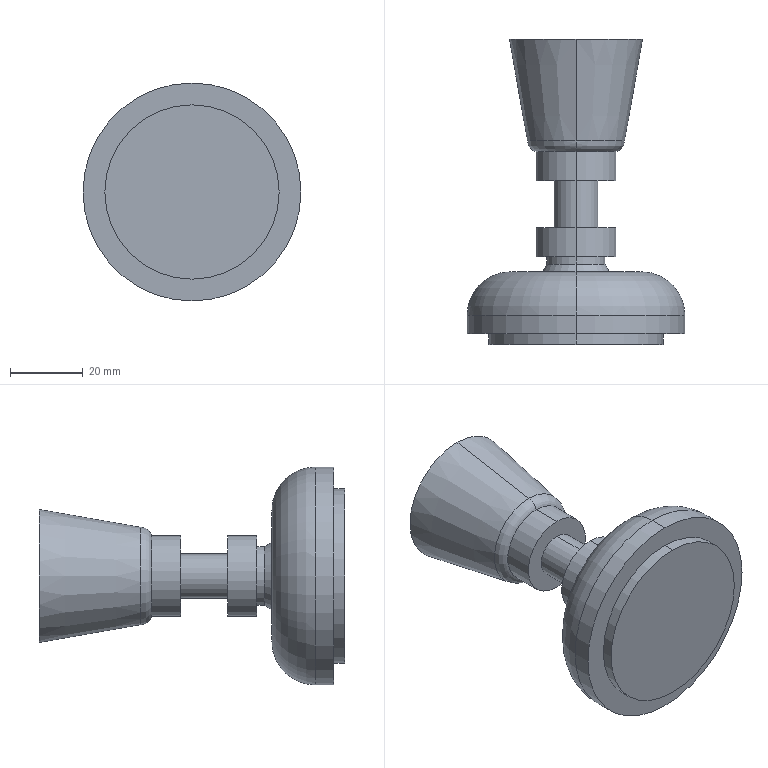Part | SolidWorks | features Revolution 1 | 1 solid | 27 faces | box 60 x 84 x 60 mm | volume 80542 mm3 | cylinder 12 | plane 7 | cone 4 | torus 4 | commonest cylinder face diameters 22.179 x4 12.179 x2 16.179 x2 48 x2 60 x2
STEP:
#1=CARTESIAN_POINT('',(0.,36.531,-13.4));
#2=VERTEX_POINT('',#1);
#3=CARTESIAN_POINT('',(0.,36.531,13.4));
#4=VERTEX_POINT('',#3);
#5=CARTESIAN_POINT('',(0.,36.531,0.));
#6=DIRECTION('',(0.,-1.,0.));
#7=DIRECTION('',(0.,0.,-1.));
#8=AXIS2_PLACEMENT_3D('',#5,#6,#7);
#9=CIRCLE('',#8,13.4);
#10=EDGE_CURVE('',#2,#4,#9,.T.);
#11=ORIENTED_EDGE('',*,*,#10,.F.);
#12=CARTESIAN_POINT('',(0.,64.484,-18.3));
#13=VERTEX_POINT('',#12);
#14=CARTESIAN_POINT('',(0.,36.531,-13.4));
#15=DIRECTION('',(0.,0.985,-0.1727));
#16=VECTOR('',#15,1000.);
#17=LINE('',#14,#16);
#18=EDGE_CURVE('',#2,#13,#17,.T.);
#19=ORIENTED_EDGE('',*,*,#18,.T.);
#20=CARTESIAN_POINT('',(0.,64.484,18.3));
#21=VERTEX_POINT('',#20);
#22=CARTESIAN_POINT('',(0.,64.484,0.));
#23=DIRECTION('',(0.,-1.,0.));
#24=DIRECTION('',(0.,0.,-1.));
#25=AXIS2_PLACEMENT_3D('',#22,#23,#24);
#26=CIRCLE('',#25,18.3);
#27=EDGE_CURVE('',#13,#21,#26,.T.);
#28=ORIENTED_EDGE('',*,*,#27,.T.);
#29=CARTESIAN_POINT('',(0.,36.531,13.4));
#30=DIRECTION('',(0.,0.985,0.1727));
#31=VECTOR('',#30,1000.);
#32=LINE('',#29,#31);
#33=EDGE_CURVE('',#4,#21,#32,.T.);
#34=ORIENTED_EDGE('',*,*,#33,.F.);
#35=EDGE_LOOP('',(#11,#19,#28,#34));
#36=FACE_OUTER_BOUND('',#35,.T.);
#37=CARTESIAN_POINT('',(0.,36.531,0.));
#38=DIRECTION('',(0.,1.,0.));
#39=DIRECTION('',(0.,0.,1.));
#40=AXIS2_PLACEMENT_3D('',#37,#38,#39);
#41=CONICAL_SURFACE('',#40,13.4,0.1735);
#42=ADVANCED_FACE('',(#36),#41,.T.);
#43=ORIENTED_EDGE('',*,*,#10,.T.);
#44=CARTESIAN_POINT('',(0.,33.612,11.09));
#45=VERTEX_POINT('',#44);
#46=CARTESIAN_POINT('',(0.,36.531,10.4));
#47=DIRECTION('',(1.,0.,0.));
#48=DIRECTION('',(0.,0.,-1.));
#49=AXIS2_PLACEMENT_3D('',#46,#47,#48);
#50=CIRCLE('',#49,3.);
#51=EDGE_CURVE('',#4,#45,#50,.T.);
#52=ORIENTED_EDGE('',*,*,#51,.T.);
#53=CARTESIAN_POINT('',(0.,33.612,-11.09));
#54=VERTEX_POINT('',#53);
#55=CARTESIAN_POINT('',(0.,33.612,0.));
#56=DIRECTION('',(0.,-1.,0.));
#57=DIRECTION('',(0.,0.,-1.));
#58=AXIS2_PLACEMENT_3D('',#55,#56,#57);
#59=CIRCLE('',#58,11.09);
#60=EDGE_CURVE('',#54,#45,#59,.T.);
#61=ORIENTED_EDGE('',*,*,#60,.F.);
#62=CARTESIAN_POINT('',(0.,36.531,-10.4));
#63=DIRECTION('',(-1.,0.,0.));
#64=DIRECTION('',(0.,0.,1.));
#65=AXIS2_PLACEMENT_3D('',#62,#63,#64);
#66=CIRCLE('',#65,3.);
#67=EDGE_CURVE('',#2,#54,#66,.T.);
#68=ORIENTED_EDGE('',*,*,#67,.F.);
#69=EDGE_LOOP('',(#43,#52,#61,#68));
#70=FACE_OUTER_BOUND('',#69,.T.);
#71=CARTESIAN_POINT('',(0.,36.531,0.));
#72=DIRECTION('',(0.,-1.,0.));
#73=DIRECTION('',(0.,0.,-1.));
#74=AXIS2_PLACEMENT_3D('',#71,#72,#73);
#75=TOROIDAL_SURFACE('',#74,10.4,3.);
#76=ADVANCED_FACE('',(#70),#75,.T.);
#77=ORIENTED_EDGE('',*,*,#60,.T.);
#78=CARTESIAN_POINT('',(0.,25.612,11.09));
#79=VERTEX_POINT('',#78);
#80=CARTESIAN_POINT('',(0.,0.,11.09));
#81=DIRECTION('',(0.,-1.,0.));
#82=VECTOR('',#81,1000.);
#83=LINE('',#80,#82);
#84=EDGE_CURVE('',#45,#79,#83,.T.);
#85=ORIENTED_EDGE('',*,*,#84,.T.);
#86=CARTESIAN_POINT('',(0.,25.612,-11.09));
#87=VERTEX_POINT('',#86);
#88=CARTESIAN_POINT('',(0.,25.612,0.));
#89=DIRECTION('',(0.,-1.,0.));
#90=DIRECTION('',(0.,0.,-1.));
#91=AXIS2_PLACEMENT_3D('',#88,#89,#90);
#92=CIRCLE('',#91,11.09);
#93=EDGE_CURVE('',#87,#79,#92,.T.);
#94=ORIENTED_EDGE('',*,*,#93,.F.);
#95=CARTESIAN_POINT('',(0.,0.,-11.09));
#96=DIRECTION('',(0.,-1.,0.));
#97=VECTOR('',#96,1000.);
#98=LINE('',#95,#97);
#99=EDGE_CURVE('',#54,#87,#98,.T.);
#100=ORIENTED_EDGE('',*,*,#99,.F.);
#101=EDGE_LOOP('',(#77,#85,#94,#100));
#102=FACE_OUTER_BOUND('',#101,.T.);
#103=CARTESIAN_POINT('',(0.,0.,0.));
#104=DIRECTION('',(0.,-1.,0.));
#105=DIRECTION('',(0.,0.,-1.));
#106=AXIS2_PLACEMENT_3D('',#103,#104,#105);
#107=CYLINDRICAL_SURFACE('',#106,11.09);
#108=ADVANCED_FACE('',(#102),#107,.T.);
#109=CARTESIAN_POINT('',(0.,25.612,-6.09));
#110=VERTEX_POINT('',#109);
#111=CARTESIAN_POINT('',(0.,25.612,6.09));
#112=VERTEX_POINT('',#111);
#113=CARTESIAN_POINT('',(0.,25.612,0.));
#114=DIRECTION('',(0.,-1.,0.));
#115=DIRECTION('',(0.,0.,-1.));
#116=AXIS2_PLACEMENT_3D('',#113,#114,#115);
#117=CIRCLE('',#116,6.09);
#118=EDGE_CURVE('',#110,#112,#117,.T.);
#119=ORIENTED_EDGE('',*,*,#118,.T.);
#120=CARTESIAN_POINT('',(0.,12.612,6.09));
#121=VERTEX_POINT('',#120);
#122=CARTESIAN_POINT('',(0.,0.,6.09));
#123=DIRECTION('',(0.,-1.,0.));
#124=VECTOR('',#123,1000.);
#125=LINE('',#122,#124);
#126=EDGE_CURVE('',#112,#121,#125,.T.);
#127=ORIENTED_EDGE('',*,*,#126,.T.);
#128=CARTESIAN_POINT('',(0.,12.612,-6.09));
#129=VERTEX_POINT('',#128);
#130=CARTESIAN_POINT('',(0.,12.612,0.));
#131=DIRECTION('',(0.,-1.,0.));
#132=DIRECTION('',(0.,0.,-1.));
#133=AXIS2_PLACEMENT_3D('',#130,#131,#132);
#134=CIRCLE('',#133,6.09);
#135=EDGE_CURVE('',#129,#121,#134,.T.);
#136=ORIENTED_EDGE('',*,*,#135,.F.);
#137=CARTESIAN_POINT('',(0.,0.,-6.09));
#138=DIRECTION('',(0.,-1.,0.));
#139=VECTOR('',#138,1000.);
#140=LINE('',#137,#139);
#141=EDGE_CURVE('',#110,#129,#140,.T.);
#142=ORIENTED_EDGE('',*,*,#141,.F.);
#143=EDGE_LOOP('',(#119,#127,#136,#142));
#144=FACE_OUTER_BOUND('',#143,.T.);
#145=CARTESIAN_POINT('',(0.,0.,0.));
#146=DIRECTION('',(0.,-1.,0.));
#147=DIRECTION('',(0.,0.,-1.));
#148=AXIS2_PLACEMENT_3D('',#145,#146,#147);
#149=CYLINDRICAL_SURFACE('',#148,6.09);
#150=ADVANCED_FACE('',(#144),#149,.T.);
#151=CARTESIAN_POINT('',(0.,12.612,-11.09));
#152=VERTEX_POINT('',#151);
#153=CARTESIAN_POINT('',(0.,12.612,11.09));
#154=VERTEX_POINT('',#153);
#155=CARTESIAN_POINT('',(0.,12.612,0.));
#156=DIRECTION('',(0.,-1.,0.));
#157=DIRECTION('',(0.,0.,-1.));
#158=AXIS2_PLACEMENT_3D('',#155,#156,#157);
#159=CIRCLE('',#158,11.09);
#160=EDGE_CURVE('',#152,#154,#159,.T.);
#161=ORIENTED_EDGE('',*,*,#160,.T.);
#162=CARTESIAN_POINT('',(0.,4.612,11.09));
#163=VERTEX_POINT('',#162);
#164=CARTESIAN_POINT('',(0.,0.,11.09));
#165=DIRECTION('',(0.,-1.,0.));
#166=VECTOR('',#165,1000.);
#167=LINE('',#164,#166);
#168=EDGE_CURVE('',#154,#163,#167,.T.);
#169=ORIENTED_EDGE('',*,*,#168,.T.);
#170=CARTESIAN_POINT('',(0.,4.612,-11.09));
#171=VERTEX_POINT('',#170);
#172=CARTESIAN_POINT('',(0.,4.612,0.));
#173=DIRECTION('',(0.,-1.,0.));
#174=DIRECTION('',(0.,0.,-1.));
#175=AXIS2_PLACEMENT_3D('',#172,#173,#174);
#176=CIRCLE('',#175,11.09);
#177=EDGE_CURVE('',#171,#163,#176,.T.);
#178=ORIENTED_EDGE('',*,*,#177,.F.);
#179=CARTESIAN_POINT('',(0.,0.,-11.09));
#180=DIRECTION('',(0.,-1.,0.));
#181=VECTOR('',#180,1000.);
#182=LINE('',#179,#181);
#183=EDGE_CURVE('',#152,#171,#182,.T.);
#184=ORIENTED_EDGE('',*,*,#183,.F.);
#185=EDGE_LOOP('',(#161,#169,#178,#184));
#186=FACE_OUTER_BOUND('',#185,.T.);
#187=CARTESIAN_POINT('',(0.,0.,0.));
#188=DIRECTION('',(0.,-1.,0.));
#189=DIRECTION('',(0.,0.,-1.));
#190=AXIS2_PLACEMENT_3D('',#187,#188,#189);
#191=CYLINDRICAL_SURFACE('',#190,11.09);
#192=ADVANCED_FACE('',(#186),#191,.T.);
#193=CARTESIAN_POINT('',(0.,4.612,-8.09));
#194=VERTEX_POINT('',#193);
#195=CARTESIAN_POINT('',(0.,4.612,8.09));
#196=VERTEX_POINT('',#195);
#197=CARTESIAN_POINT('',(0.,4.612,0.));
#198=DIRECTION('',(0.,-1.,0.));
#199=DIRECTION('',(0.,0.,-1.));
#200=AXIS2_PLACEMENT_3D('',#197,#198,#199);
#201=CIRCLE('',#200,8.09);
#202=EDGE_CURVE('',#194,#196,#201,.T.);
#203=ORIENTED_EDGE('',*,*,#202,.T.);
#204=CARTESIAN_POINT('',(0.,2.612,8.09));
#205=VERTEX_POINT('',#204);
#206=CARTESIAN_POINT('',(0.,0.,8.09));
#207=DIRECTION('',(0.,-1.,0.));
#208=VECTOR('',#207,1000.);
#209=LINE('',#206,#208);
#210=EDGE_CURVE('',#196,#205,#209,.T.);
#211=ORIENTED_EDGE('',*,*,#210,.T.);
#212=CARTESIAN_POINT('',(0.,2.612,-8.09));
#213=VERTEX_POINT('',#212);
#214=CARTESIAN_POINT('',(0.,2.612,0.));
#215=DIRECTION('',(0.,-1.,0.));
#216=DIRECTION('',(0.,0.,-1.));
#217=AXIS2_PLACEMENT_3D('',#214,#215,#216);
#218=CIRCLE('',#217,8.09);
#219=EDGE_CURVE('',#213,#205,#218,.T.);
#220=ORIENTED_EDGE('',*,*,#219,.F.);
#221=CARTESIAN_POINT('',(0.,0.,-8.09));
#222=DIRECTION('',(0.,-1.,0.));
#223=VECTOR('',#222,1000.);
#224=LINE('',#221,#223);
#225=EDGE_CURVE('',#194,#213,#224,.T.);
#226=ORIENTED_EDGE('',*,*,#225,.F.);
#227=EDGE_LOOP('',(#203,#211,#220,#226));
#228=FACE_OUTER_BOUND('',#227,.T.);
#229=CARTESIAN_POINT('',(0.,0.,0.));
#230=DIRECTION('',(0.,-1.,0.));
#231=DIRECTION('',(0.,0.,-1.));
#232=AXIS2_PLACEMENT_3D('',#229,#230,#231);
#233=CYLINDRICAL_SURFACE('',#232,8.09);
#234=ADVANCED_FACE('',(#228),#233,.T.);
#235=ORIENTED_EDGE('',*,*,#219,.T.);
#236=CARTESIAN_POINT('',(0.,0.4839,9.2));
#237=VERTEX_POINT('',#236);
#238=CARTESIAN_POINT('',(0.,0.4839,9.2));
#239=DIRECTION('',(0.,-0.8865,0.4627));
#240=VECTOR('',#239,1000.);
#241=LINE('',#238,#240);
#242=EDGE_CURVE('',#205,#237,#241,.T.);
#243=ORIENTED_EDGE('',*,*,#242,.T.);
#244=CARTESIAN_POINT('',(0.,0.4839,-9.2));
#245=VERTEX_POINT('',#244);
#246=CARTESIAN_POINT('',(0.,0.4839,0.));
#247=DIRECTION('',(0.,-1.,0.));
#248=DIRECTION('',(0.,0.,-1.));
#249=AXIS2_PLACEMENT_3D('',#246,#247,#248);
#250=CIRCLE('',#249,9.2);
#251=EDGE_CURVE('',#245,#237,#250,.T.);
#252=ORIENTED_EDGE('',*,*,#251,.F.);
#253=CARTESIAN_POINT('',(0.,0.4839,-9.2));
#254=DIRECTION('',(0.,-0.8865,-0.4627));
#255=VECTOR('',#254,1000.);
#256=LINE('',#253,#255);
#257=EDGE_CURVE('',#213,#245,#256,.T.);
#258=ORIENTED_EDGE('',*,*,#257,.F.);
#259=EDGE_LOOP('',(#235,#243,#252,#258));
#260=FACE_OUTER_BOUND('',#259,.T.);
#261=CARTESIAN_POINT('',(0.,0.4839,0.));
#262=DIRECTION('',(0.,-1.,0.));
#263=DIRECTION('',(0.,0.,-1.));
#264=AXIS2_PLACEMENT_3D('',#261,#262,#263);
#265=CONICAL_SURFACE('',#264,9.2,0.481);
#266=ADVANCED_FACE('',(#260),#265,.T.);
#267=CARTESIAN_POINT('',(0.,0.4839,-18.));
#268=VERTEX_POINT('',#267);
#269=CARTESIAN_POINT('',(0.,0.4839,18.));
#270=VERTEX_POINT('',#269);
#271=CARTESIAN_POINT('',(0.,0.4839,0.));
#272=DIRECTION('',(0.,-1.,0.));
#273=DIRECTION('',(0.,0.,-1.));
#274=AXIS2_PLACEMENT_3D('',#271,#272,#273);
#275=CIRCLE('',#274,18.);
#276=EDGE_CURVE('',#268,#270,#275,.T.);
#277=ORIENTED_EDGE('',*,*,#276,.T.);
#278=CARTESIAN_POINT('',(0.,-11.516,30.));
#279=VERTEX_POINT('',#278);
#280=CARTESIAN_POINT('',(0.,-11.516,18.));
#281=DIRECTION('',(1.,0.,0.));
#282=DIRECTION('',(0.,0.,-1.));
#283=AXIS2_PLACEMENT_3D('',#280,#281,#282);
#284=CIRCLE('',#283,12.);
#285=EDGE_CURVE('',#270,#279,#284,.T.);
#286=ORIENTED_EDGE('',*,*,#285,.T.);
#287=CARTESIAN_POINT('',(0.,-11.516,-30.));
#288=VERTEX_POINT('',#287);
#289=CARTESIAN_POINT('',(0.,-11.516,0.));
#290=DIRECTION('',(0.,-1.,0.));
#291=DIRECTION('',(0.,0.,-1.));
#292=AXIS2_PLACEMENT_3D('',#289,#290,#291);
#293=CIRCLE('',#292,30.);
#294=EDGE_CURVE('',#288,#279,#293,.T.);
#295=ORIENTED_EDGE('',*,*,#294,.F.);
#296=CARTESIAN_POINT('',(0.,-11.516,-18.));
#297=DIRECTION('',(-1.,0.,0.));
#298=DIRECTION('',(0.,0.,1.));
#299=AXIS2_PLACEMENT_3D('',#296,#297,#298);
#300=CIRCLE('',#299,12.);
#301=EDGE_CURVE('',#268,#288,#300,.T.);
#302=ORIENTED_EDGE('',*,*,#301,.F.);
#303=EDGE_LOOP('',(#277,#286,#295,#302));
#304=FACE_OUTER_BOUND('',#303,.T.);
#305=CARTESIAN_POINT('',(0.,-11.516,0.));
#306=DIRECTION('',(0.,-1.,0.));
#307=DIRECTION('',(0.,0.,-1.));
#308=AXIS2_PLACEMENT_3D('',#305,#306,#307);
#309=TOROIDAL_SURFACE('',#308,18.,12.);
#310=ADVANCED_FACE('',(#304),#309,.T.);
#311=ORIENTED_EDGE('',*,*,#294,.T.);
#312=CARTESIAN_POINT('',(0.,-16.516,30.));
#313=VERTEX_POINT('',#312);
#314=CARTESIAN_POINT('',(0.,0.,30.));
#315=DIRECTION('',(0.,-1.,0.));
#316=VECTOR('',#315,1000.);
#317=LINE('',#314,#316);
#318=EDGE_CURVE('',#279,#313,#317,.T.);
#319=ORIENTED_EDGE('',*,*,#318,.T.);
#320=CARTESIAN_POINT('',(0.,-16.516,-30.));
#321=VERTEX_POINT('',#320);
#322=CARTESIAN_POINT('',(0.,-16.516,0.));
#323=DIRECTION('',(0.,-1.,0.));
#324=DIRECTION('',(0.,0.,-1.));
#325=AXIS2_PLACEMENT_3D('',#322,#323,#324);
#326=CIRCLE('',#325,30.);
#327=EDGE_CURVE('',#321,#313,#326,.T.);
#328=ORIENTED_EDGE('',*,*,#327,.F.);
#329=CARTESIAN_POINT('',(0.,0.,-30.));
#330=DIRECTION('',(0.,-1.,0.));
#331=VECTOR('',#330,1000.);
#332=LINE('',#329,#331);
#333=EDGE_CURVE('',#288,#321,#332,.T.);
#334=ORIENTED_EDGE('',*,*,#333,.F.);
#335=EDGE_LOOP('',(#311,#319,#328,#334));
#336=FACE_OUTER_BOUND('',#335,.T.);
#337=CARTESIAN_POINT('',(0.,0.,0.));
#338=DIRECTION('',(0.,-1.,0.));
#339=DIRECTION('',(0.,0.,-1.));
#340=AXIS2_PLACEMENT_3D('',#337,#338,#339);
#341=CYLINDRICAL_SURFACE('',#340,30.);
#342=ADVANCED_FACE('',(#336),#341,.T.);
#343=CARTESIAN_POINT('',(0.,-16.516,-24.));
#344=VERTEX_POINT('',#343);
#345=CARTESIAN_POINT('',(0.,-16.516,24.));
#346=VERTEX_POINT('',#345);
#347=CARTESIAN_POINT('',(0.,-16.516,0.));
#348=DIRECTION('',(0.,-1.,0.));
#349=DIRECTION('',(0.,0.,-1.));
#350=AXIS2_PLACEMENT_3D('',#347,#348,#349);
#351=CIRCLE('',#350,24.);
#352=EDGE_CURVE('',#344,#346,#351,.T.);
#353=ORIENTED_EDGE('',*,*,#352,.T.);
#354=CARTESIAN_POINT('',(0.,-19.516,24.));
#355=VERTEX_POINT('',#354);
#356=CARTESIAN_POINT('',(0.,0.,24.));
#357=DIRECTION('',(0.,-1.,0.));
#358=VECTOR('',#357,1000.);
#359=LINE('',#356,#358);
#360=EDGE_CURVE('',#346,#355,#359,.T.);
#361=ORIENTED_EDGE('',*,*,#360,.T.);
#362=CARTESIAN_POINT('',(0.,-19.516,-24.));
#363=VERTEX_POINT('',#362);
#364=CARTESIAN_POINT('',(0.,-19.516,0.));
#365=DIRECTION('',(0.,-1.,0.));
#366=DIRECTION('',(0.,0.,-1.));
#367=AXIS2_PLACEMENT_3D('',#364,#365,#366);
#368=CIRCLE('',#367,24.);
#369=EDGE_CURVE('',#363,#355,#368,.T.);
#370=ORIENTED_EDGE('',*,*,#369,.F.);
#371=CARTESIAN_POINT('',(0.,0.,-24.));
#372=DIRECTION('',(0.,-1.,0.));
#373=VECTOR('',#372,1000.);
#374=LINE('',#371,#373);
#375=EDGE_CURVE('',#344,#363,#374,.T.);
#376=ORIENTED_EDGE('',*,*,#375,.F.);
#377=EDGE_LOOP('',(#353,#361,#370,#376));
#378=FACE_OUTER_BOUND('',#377,.T.);
#379=CARTESIAN_POINT('',(0.,0.,0.));
#380=DIRECTION('',(0.,-1.,0.));
#381=DIRECTION('',(0.,0.,-1.));
#382=AXIS2_PLACEMENT_3D('',#379,#380,#381);
#383=CYLINDRICAL_SURFACE('',#382,24.);
#384=ADVANCED_FACE('',(#378),#383,.T.);
#385=ORIENTED_EDGE('',*,*,#369,.T.);
#386=CARTESIAN_POINT('',(0.,-19.516,0.));
#387=DIRECTION('',(0.,-1.,0.));
#388=DIRECTION('',(0.,0.,-1.));
#389=AXIS2_PLACEMENT_3D('',#386,#387,#388);
#390=CIRCLE('',#389,24.);
#391=EDGE_CURVE('',#355,#363,#390,.T.);
#392=ORIENTED_EDGE('',*,*,#391,.T.);
#393=EDGE_LOOP('',(#385,#392));
#394=FACE_OUTER_BOUND('',#393,.T.);
#395=CARTESIAN_POINT('',(0.,-19.516,0.));
#396=DIRECTION('',(0.,-1.,0.));
#397=DIRECTION('',(0.,0.,-1.));
#398=AXIS2_PLACEMENT_3D('',#395,#396,#397);
#399=PLANE('',#398);
#400=ADVANCED_FACE('',(#394),#399,.T.);
#401=ORIENTED_EDGE('',*,*,#360,.F.);
#402=CARTESIAN_POINT('',(0.,-16.516,0.));
#403=DIRECTION('',(0.,-1.,0.));
#404=DIRECTION('',(0.,0.,-1.));
#405=AXIS2_PLACEMENT_3D('',#402,#403,#404);
#406=CIRCLE('',#405,24.);
#407=EDGE_CURVE('',#346,#344,#406,.T.);
#408=ORIENTED_EDGE('',*,*,#407,.T.);
#409=ORIENTED_EDGE('',*,*,#375,.T.);
#410=ORIENTED_EDGE('',*,*,#391,.F.);
#411=EDGE_LOOP('',(#401,#408,#409,#410));
#412=FACE_OUTER_BOUND('',#411,.T.);
#413=CARTESIAN_POINT('',(0.,0.,0.));
#414=DIRECTION('',(0.,-1.,0.));
#415=DIRECTION('',(0.,0.,-1.));
#416=AXIS2_PLACEMENT_3D('',#413,#414,#415);
#417=CYLINDRICAL_SURFACE('',#416,24.);
#418=ADVANCED_FACE('',(#412),#417,.T.);
#419=ORIENTED_EDGE('',*,*,#327,.T.);
#420=CARTESIAN_POINT('',(0.,-16.516,0.));
#421=DIRECTION('',(0.,-1.,0.));
#422=DIRECTION('',(0.,0.,-1.));
#423=AXIS2_PLACEMENT_3D('',#420,#421,#422);
#424=CIRCLE('',#423,30.);
#425=EDGE_CURVE('',#313,#321,#424,.T.);
#426=ORIENTED_EDGE('',*,*,#425,.T.);
#427=EDGE_LOOP('',(#419,#426));
#428=FACE_OUTER_BOUND('',#427,.T.);
#429=ORIENTED_EDGE('',*,*,#352,.F.);
#430=ORIENTED_EDGE('',*,*,#407,.F.);
#431=EDGE_LOOP('',(#429,#430));
#432=FACE_BOUND('',#431,.T.);
#433=CARTESIAN_POINT('',(24.,-16.516,0.));
#434=DIRECTION('',(0.,-1.,0.));
#435=DIRECTION('',(0.,0.,-1.));
#436=AXIS2_PLACEMENT_3D('',#433,#434,#435);
#437=PLANE('',#436);
#438=ADVANCED_FACE('',(#428,#432),#437,.T.);
#439=ORIENTED_EDGE('',*,*,#318,.F.);
#440=CARTESIAN_POINT('',(0.,-11.516,0.));
#441=DIRECTION('',(0.,-1.,0.));
#442=DIRECTION('',(0.,0.,-1.));
#443=AXIS2_PLACEMENT_3D('',#440,#441,#442);
#444=CIRCLE('',#443,30.);
#445=EDGE_CURVE('',#279,#288,#444,.T.);
#446=ORIENTED_EDGE('',*,*,#445,.T.);
#447=ORIENTED_EDGE('',*,*,#333,.T.);
#448=ORIENTED_EDGE('',*,*,#425,.F.);
#449=EDGE_LOOP('',(#439,#446,#447,#448));
#450=FACE_OUTER_BOUND('',#449,.T.);
#451=CARTESIAN_POINT('',(0.,0.,0.));
#452=DIRECTION('',(0.,-1.,0.));
#453=DIRECTION('',(0.,0.,-1.));
#454=AXIS2_PLACEMENT_3D('',#451,#452,#453);
#455=CYLINDRICAL_SURFACE('',#454,30.);
#456=ADVANCED_FACE('',(#450),#455,.T.);
#457=ORIENTED_EDGE('',*,*,#285,.F.);
#458=CARTESIAN_POINT('',(0.,0.4839,0.));
#459=DIRECTION('',(0.,-1.,0.));
#460=DIRECTION('',(0.,0.,-1.));
#461=AXIS2_PLACEMENT_3D('',#458,#459,#460);
#462=CIRCLE('',#461,18.);
#463=EDGE_CURVE('',#270,#268,#462,.T.);
#464=ORIENTED_EDGE('',*,*,#463,.T.);
#465=ORIENTED_EDGE('',*,*,#301,.T.);
#466=ORIENTED_EDGE('',*,*,#445,.F.);
#467=EDGE_LOOP('',(#457,#464,#465,#466));
#468=FACE_OUTER_BOUND('',#467,.T.);
#469=CARTESIAN_POINT('',(0.,-11.516,0.));
#470=DIRECTION('',(0.,-1.,0.));
#471=DIRECTION('',(0.,0.,-1.));
#472=AXIS2_PLACEMENT_3D('',#469,#470,#471);
#473=TOROIDAL_SURFACE('',#472,18.,12.);
#474=ADVANCED_FACE('',(#468),#473,.T.);
#475=ORIENTED_EDGE('',*,*,#251,.T.);
#476=CARTESIAN_POINT('',(0.,0.4839,0.));
#477=DIRECTION('',(0.,-1.,0.));
#478=DIRECTION('',(0.,0.,-1.));
#479=AXIS2_PLACEMENT_3D('',#476,#477,#478);
#480=CIRCLE('',#479,9.2);
#481=EDGE_CURVE('',#237,#245,#480,.T.);
#482=ORIENTED_EDGE('',*,*,#481,.T.);
#483=EDGE_LOOP('',(#475,#482));
#484=FACE_BOUND('',#483,.T.);
#485=ORIENTED_EDGE('',*,*,#276,.F.);
#486=ORIENTED_EDGE('',*,*,#463,.F.);
#487=EDGE_LOOP('',(#485,#486));
#488=FACE_OUTER_BOUND('',#487,.T.);
#489=CARTESIAN_POINT('',(18.,0.4839,0.));
#490=DIRECTION('',(0.,1.,0.));
#491=DIRECTION('',(0.,0.,1.));
#492=AXIS2_PLACEMENT_3D('',#489,#490,#491);
#493=PLANE('',#492);
#494=ADVANCED_FACE('',(#484,#488),#493,.T.);
#495=ORIENTED_EDGE('',*,*,#242,.F.);
#496=CARTESIAN_POINT('',(0.,2.612,0.));
#497=DIRECTION('',(0.,-1.,0.));
#498=DIRECTION('',(0.,0.,-1.));
#499=AXIS2_PLACEMENT_3D('',#496,#497,#498);
#500=CIRCLE('',#499,8.09);
#501=EDGE_CURVE('',#205,#213,#500,.T.);
#502=ORIENTED_EDGE('',*,*,#501,.T.);
#503=ORIENTED_EDGE('',*,*,#257,.T.);
#504=ORIENTED_EDGE('',*,*,#481,.F.);
#505=EDGE_LOOP('',(#495,#502,#503,#504));
#506=FACE_OUTER_BOUND('',#505,.T.);
#507=CARTESIAN_POINT('',(0.,0.4839,0.));
#508=DIRECTION('',(0.,-1.,0.));
#509=DIRECTION('',(0.,0.,-1.));
#510=AXIS2_PLACEMENT_3D('',#507,#508,#509);
#511=CONICAL_SURFACE('',#510,9.2,0.481);
#512=ADVANCED_FACE('',(#506),#511,.T.);
#513=ORIENTED_EDGE('',*,*,#210,.F.);
#514=CARTESIAN_POINT('',(0.,4.612,0.));
#515=DIRECTION('',(0.,-1.,0.));
#516=DIRECTION('',(0.,0.,-1.));
#517=AXIS2_PLACEMENT_3D('',#514,#515,#516);
#518=CIRCLE('',#517,8.09);
#519=EDGE_CURVE('',#196,#194,#518,.T.);
#520=ORIENTED_EDGE('',*,*,#519,.T.);
#521=ORIENTED_EDGE('',*,*,#225,.T.);
#522=ORIENTED_EDGE('',*,*,#501,.F.);
#523=EDGE_LOOP('',(#513,#520,#521,#522));
#524=FACE_OUTER_BOUND('',#523,.T.);
#525=CARTESIAN_POINT('',(0.,0.,0.));
#526=DIRECTION('',(0.,-1.,0.));
#527=DIRECTION('',(0.,0.,-1.));
#528=AXIS2_PLACEMENT_3D('',#525,#526,#527);
#529=CYLINDRICAL_SURFACE('',#528,8.09);
#530=ADVANCED_FACE('',(#524),#529,.T.);
#531=ORIENTED_EDGE('',*,*,#177,.T.);
#532=CARTESIAN_POINT('',(0.,4.612,0.));
#533=DIRECTION('',(0.,-1.,0.));
#534=DIRECTION('',(0.,0.,-1.));
#535=AXIS2_PLACEMENT_3D('',#532,#533,#534);
#536=CIRCLE('',#535,11.09);
#537=EDGE_CURVE('',#163,#171,#536,.T.);
#538=ORIENTED_EDGE('',*,*,#537,.T.);
#539=EDGE_LOOP('',(#531,#538));
#540=FACE_OUTER_BOUND('',#539,.T.);
#541=ORIENTED_EDGE('',*,*,#202,.F.);
#542=ORIENTED_EDGE('',*,*,#519,.F.);
#543=EDGE_LOOP('',(#541,#542));
#544=FACE_BOUND('',#543,.T.);
#545=CARTESIAN_POINT('',(8.09,4.612,0.));
#546=DIRECTION('',(0.,-1.,0.));
#547=DIRECTION('',(0.,0.,-1.));
#548=AXIS2_PLACEMENT_3D('',#545,#546,#547);
#549=PLANE('',#548);
#550=ADVANCED_FACE('',(#540,#544),#549,.T.);
#551=ORIENTED_EDGE('',*,*,#168,.F.);
#552=CARTESIAN_POINT('',(0.,12.612,0.));
#553=DIRECTION('',(0.,-1.,0.));
#554=DIRECTION('',(0.,0.,-1.));
#555=AXIS2_PLACEMENT_3D('',#552,#553,#554);
#556=CIRCLE('',#555,11.09);
#557=EDGE_CURVE('',#154,#152,#556,.T.);
#558=ORIENTED_EDGE('',*,*,#557,.T.);
#559=ORIENTED_EDGE('',*,*,#183,.T.);
#560=ORIENTED_EDGE('',*,*,#537,.F.);
#561=EDGE_LOOP('',(#551,#558,#559,#560));
#562=FACE_OUTER_BOUND('',#561,.T.);
#563=CARTESIAN_POINT('',(0.,0.,0.));
#564=DIRECTION('',(0.,-1.,0.));
#565=DIRECTION('',(0.,0.,-1.));
#566=AXIS2_PLACEMENT_3D('',#563,#564,#565);
#567=CYLINDRICAL_SURFACE('',#566,11.09);
#568=ADVANCED_FACE('',(#562),#567,.T.);
#569=ORIENTED_EDGE('',*,*,#135,.T.);
#570=CARTESIAN_POINT('',(0.,12.612,0.));
#571=DIRECTION('',(0.,-1.,0.));
#572=DIRECTION('',(0.,0.,-1.));
#573=AXIS2_PLACEMENT_3D('',#570,#571,#572);
#574=CIRCLE('',#573,6.09);
#575=EDGE_CURVE('',#121,#129,#574,.T.);
#576=ORIENTED_EDGE('',*,*,#575,.T.);
#577=EDGE_LOOP('',(#569,#576));
#578=FACE_BOUND('',#577,.T.);
#579=ORIENTED_EDGE('',*,*,#160,.F.);
#580=ORIENTED_EDGE('',*,*,#557,.F.);
#581=EDGE_LOOP('',(#579,#580));
#582=FACE_OUTER_BOUND('',#581,.T.);
#583=CARTESIAN_POINT('',(11.09,12.612,0.));
#584=DIRECTION('',(0.,1.,0.));
#585=DIRECTION('',(0.,0.,1.));
#586=AXIS2_PLACEMENT_3D('',#583,#584,#585);
#587=PLANE('',#586);
#588=ADVANCED_FACE('',(#578,#582),#587,.T.);
#589=ORIENTED_EDGE('',*,*,#126,.F.);
#590=CARTESIAN_POINT('',(0.,25.612,0.));
#591=DIRECTION('',(0.,-1.,0.));
#592=DIRECTION('',(0.,0.,-1.));
#593=AXIS2_PLACEMENT_3D('',#590,#591,#592);
#594=CIRCLE('',#593,6.09);
#595=EDGE_CURVE('',#112,#110,#594,.T.);
#596=ORIENTED_EDGE('',*,*,#595,.T.);
#597=ORIENTED_EDGE('',*,*,#141,.T.);
#598=ORIENTED_EDGE('',*,*,#575,.F.);
#599=EDGE_LOOP('',(#589,#596,#597,#598));
#600=FACE_OUTER_BOUND('',#599,.T.);
#601=CARTESIAN_POINT('',(0.,0.,0.));
#602=DIRECTION('',(0.,-1.,0.));
#603=DIRECTION('',(0.,0.,-1.));
#604=AXIS2_PLACEMENT_3D('',#601,#602,#603);
#605=CYLINDRICAL_SURFACE('',#604,6.09);
#606=ADVANCED_FACE('',(#600),#605,.T.);
#607=ORIENTED_EDGE('',*,*,#93,.T.);
#608=CARTESIAN_POINT('',(0.,25.612,0.));
#609=DIRECTION('',(0.,-1.,0.));
#610=DIRECTION('',(0.,0.,-1.));
#611=AXIS2_PLACEMENT_3D('',#608,#609,#610);
#612=CIRCLE('',#611,11.09);
#613=EDGE_CURVE('',#79,#87,#612,.T.);
#614=ORIENTED_EDGE('',*,*,#613,.T.);
#615=EDGE_LOOP('',(#607,#614));
#616=FACE_OUTER_BOUND('',#615,.T.);
#617=ORIENTED_EDGE('',*,*,#118,.F.);
#618=ORIENTED_EDGE('',*,*,#595,.F.);
#619=EDGE_LOOP('',(#617,#618));
#620=FACE_BOUND('',#619,.T.);
#621=CARTESIAN_POINT('',(6.09,25.612,0.));
#622=DIRECTION('',(0.,-1.,0.));
#623=DIRECTION('',(0.,0.,-1.));
#624=AXIS2_PLACEMENT_3D('',#621,#622,#623);
#625=PLANE('',#624);
#626=ADVANCED_FACE('',(#616,#620),#625,.T.);
#627=ORIENTED_EDGE('',*,*,#84,.F.);
#628=CARTESIAN_POINT('',(0.,33.612,0.));
#629=DIRECTION('',(0.,-1.,0.));
#630=DIRECTION('',(0.,0.,-1.));
#631=AXIS2_PLACEMENT_3D('',#628,#629,#630);
#632=CIRCLE('',#631,11.09);
#633=EDGE_CURVE('',#45,#54,#632,.T.);
#634=ORIENTED_EDGE('',*,*,#633,.T.);
#635=ORIENTED_EDGE('',*,*,#99,.T.);
#636=ORIENTED_EDGE('',*,*,#613,.F.);
#637=EDGE_LOOP('',(#627,#634,#635,#636));
#638=FACE_OUTER_BOUND('',#637,.T.);
#639=CARTESIAN_POINT('',(0.,0.,0.));
#640=DIRECTION('',(0.,-1.,0.));
#641=DIRECTION('',(0.,0.,-1.));
#642=AXIS2_PLACEMENT_3D('',#639,#640,#641);
#643=CYLINDRICAL_SURFACE('',#642,11.09);
#644=ADVANCED_FACE('',(#638),#643,.T.);
#645=ORIENTED_EDGE('',*,*,#51,.F.);
#646=CARTESIAN_POINT('',(0.,36.531,0.));
#647=DIRECTION('',(0.,-1.,0.));
#648=DIRECTION('',(0.,0.,-1.));
#649=AXIS2_PLACEMENT_3D('',#646,#647,#648);
#650=CIRCLE('',#649,13.4);
#651=EDGE_CURVE('',#4,#2,#650,.T.);
#652=ORIENTED_EDGE('',*,*,#651,.T.);
#653=ORIENTED_EDGE('',*,*,#67,.T.);
#654=ORIENTED_EDGE('',*,*,#633,.F.);
#655=EDGE_LOOP('',(#645,#652,#653,#654));
#656=FACE_OUTER_BOUND('',#655,.T.);
#657=CARTESIAN_POINT('',(0.,36.531,0.));
#658=DIRECTION('',(0.,-1.,0.));
#659=DIRECTION('',(0.,0.,-1.));
#660=AXIS2_PLACEMENT_3D('',#657,#658,#659);
#661=TOROIDAL_SURFACE('',#660,10.4,3.);
#662=ADVANCED_FACE('',(#656),#661,.T.);
#663=ORIENTED_EDGE('',*,*,#18,.F.);
#664=ORIENTED_EDGE('',*,*,#651,.F.);
#665=ORIENTED_EDGE('',*,*,#33,.T.);
#666=CARTESIAN_POINT('',(0.,64.484,0.));
#667=DIRECTION('',(0.,-1.,0.));
#668=DIRECTION('',(0.,0.,-1.));
#669=AXIS2_PLACEMENT_3D('',#666,#667,#668);
#670=CIRCLE('',#669,18.3);
#671=EDGE_CURVE('',#21,#13,#670,.T.);
#672=ORIENTED_EDGE('',*,*,#671,.T.);
#673=EDGE_LOOP('',(#663,#664,#665,#672));
#674=FACE_OUTER_BOUND('',#673,.T.);
#675=CARTESIAN_POINT('',(0.,36.531,0.));
#676=DIRECTION('',(0.,1.,0.));
#677=DIRECTION('',(0.,0.,1.));
#678=AXIS2_PLACEMENT_3D('',#675,#676,#677);
#679=CONICAL_SURFACE('',#678,13.4,0.1735);
#680=ADVANCED_FACE('',(#674),#679,.T.);
#681=ORIENTED_EDGE('',*,*,#671,.F.);
#682=ORIENTED_EDGE('',*,*,#27,.F.);
#683=EDGE_LOOP('',(#681,#682));
#684=FACE_OUTER_BOUND('',#683,.T.);
#685=CARTESIAN_POINT('',(0.,64.484,0.));
#686=DIRECTION('',(0.,1.,0.));
#687=DIRECTION('',(0.,0.,1.));
#688=AXIS2_PLACEMENT_3D('',#685,#686,#687);
#689=PLANE('',#688);
#690=ADVANCED_FACE('',(#684),#689,.T.);
#691=CLOSED_SHELL('',(#42,#76,#108,#150,#192,#234,#266,#310,#342,#384,#400,#418,#438,#456,#474,#494,#512,#530,#550,#568,#588,#606,#626,#644,#662,#680,#690));
#692=MANIFOLD_SOLID_BREP('',#691);
#693=CARTESIAN_POINT('',(0.,0.,0.));
#694=DIRECTION('',(0.,0.,1.));
#695=DIRECTION('',(1.,0.,0.));
#696=AXIS2_PLACEMENT_3D('',#693,#694,#695);
#697=(LENGTH_UNIT()NAMED_UNIT(*)SI_UNIT(.MILLI.,.METRE.));
#698=UNCERTAINTY_MEASURE_WITH_UNIT(LENGTH_MEASURE(0.00001),#697,'','');
#699=(NAMED_UNIT(*)PLANE_ANGLE_UNIT()SI_UNIT($,.RADIAN.));
#700=(NAMED_UNIT(*)SI_UNIT($,.STERADIAN.)SOLID_ANGLE_UNIT());
#701=(GEOMETRIC_REPRESENTATION_CONTEXT(3)GLOBAL_UNCERTAINTY_ASSIGNED_CONTEXT((#698))GLOBAL_UNIT_ASSIGNED_CONTEXT((#697,#699,#700))REPRESENTATION_CONTEXT('',''));
#702=ADVANCED_BREP_SHAPE_REPRESENTATION('',(#692,#696),#701);